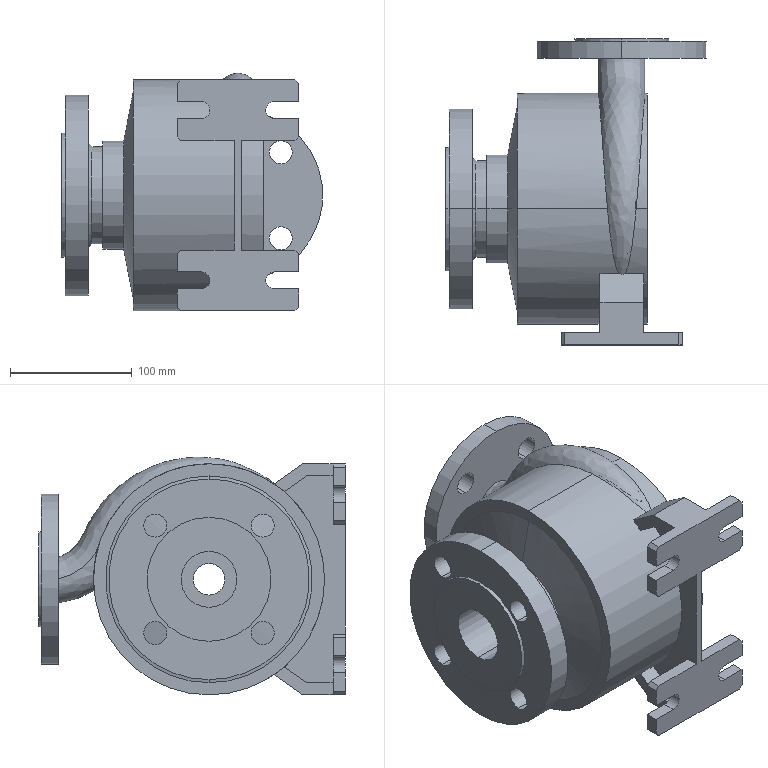Part | SolidWorks | features ICE 13, Fillet 3, Chamfer 2, Cut 2, MirrorPattern 2, Revolution 2, Blend 1, BlendCut 1, CirPattern 1, Helix 1, HoleWzd 1, MoveCopyBody 1, MoveFace 1, RevCut 1, Split 1 | 1 solid | 175 faces | box 215 x 252 x 195.497 mm | volume 2163727 mm3 | plane 78 | cylinder 71 | spline 11 | torus 9 | cone 6 | commonest cylinder face diameters 7 x20 19 x16 14 x4 190 x4 154 x3 25 x2